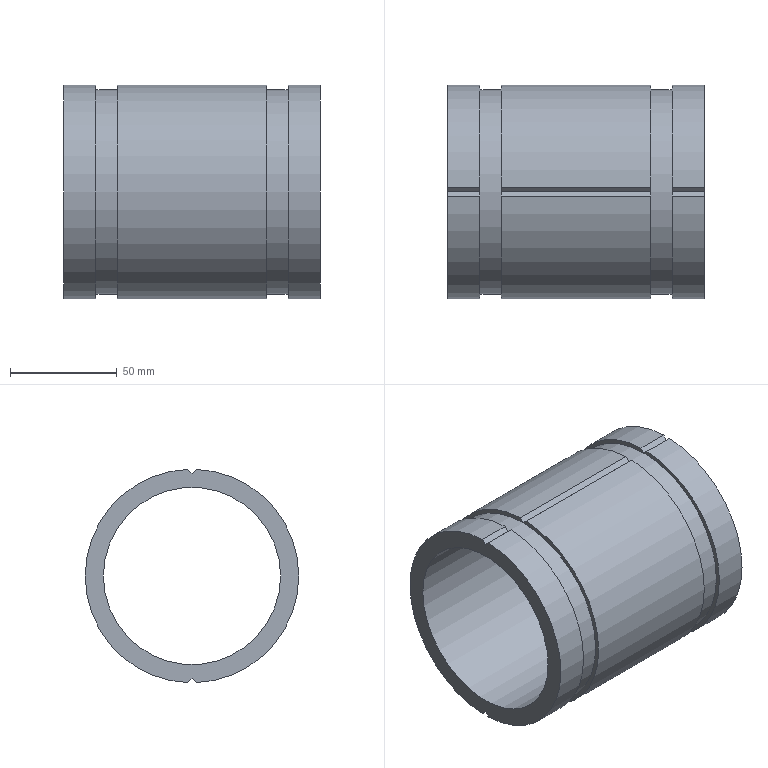Part | NX | features solid 2 | 1 solid | 31 faces | box 120 x 100 x 99.923 mm | volume 280100 mm3 | plane 22 | cylinder 9 | commonest cylinder face diameters 100 x6 96 x2 83 x1
STEP:
#1=CARTESIAN_POINT('',(1975.,798.5,-480.));
#2=VERTEX_POINT('',#1);
#3=CARTESIAN_POINT('',(1975.,840.,-480.));
#4=DIRECTION('',(-1.,0.,0.));
#5=DIRECTION('',(0.,-1.,0.));
#6=AXIS2_PLACEMENT_3D('',#3,#4,#5);
#7=CIRCLE('',#6,41.5);
#8=EDGE_CURVE('',#2,#2,#7,.T.);
#9=ORIENTED_EDGE('',*,*,#8,.T.);
#10=EDGE_LOOP('',(#9));
#11=FACE_BOUND('',#10,.T.);
#12=CARTESIAN_POINT('',(1975.,838.038,-529.962));
#13=VERTEX_POINT('',#12);
#14=CARTESIAN_POINT('',(1975.,840.,-528.));
#15=VERTEX_POINT('',#14);
#16=CARTESIAN_POINT('',(1975.,830.,-538.));
#17=DIRECTION('',(0.,0.7071,0.7071));
#18=VECTOR('',#17,1000.);
#19=LINE('',#16,#18);
#20=EDGE_CURVE('',#13,#15,#19,.T.);
#21=ORIENTED_EDGE('',*,*,#20,.T.);
#22=CARTESIAN_POINT('',(1975.,841.962,-529.962));
#23=VERTEX_POINT('',#22);
#24=CARTESIAN_POINT('',(1975.,840.,-528.));
#25=DIRECTION('',(0.,0.7071,-0.7071));
#26=VECTOR('',#25,1000.);
#27=LINE('',#24,#26);
#28=EDGE_CURVE('',#15,#23,#27,.T.);
#29=ORIENTED_EDGE('',*,*,#28,.T.);
#30=CARTESIAN_POINT('',(1975.,841.962,-430.038));
#31=VERTEX_POINT('',#30);
#32=CARTESIAN_POINT('',(1975.,840.,-480.));
#33=DIRECTION('',(-1.,0.,0.));
#34=DIRECTION('',(0.,-1.,0.));
#35=AXIS2_PLACEMENT_3D('',#32,#33,#34);
#36=CIRCLE('',#35,50.);
#37=EDGE_CURVE('',#31,#23,#36,.T.);
#38=ORIENTED_EDGE('',*,*,#37,.F.);
#39=CARTESIAN_POINT('',(1975.,840.,-432.));
#40=VERTEX_POINT('',#39);
#41=CARTESIAN_POINT('',(1975.,840.,-432.));
#42=DIRECTION('',(0.,0.7071,0.7071));
#43=VECTOR('',#42,1000.);
#44=LINE('',#41,#43);
#45=EDGE_CURVE('',#40,#31,#44,.T.);
#46=ORIENTED_EDGE('',*,*,#45,.F.);
#47=CARTESIAN_POINT('',(1975.,838.038,-430.038));
#48=VERTEX_POINT('',#47);
#49=CARTESIAN_POINT('',(1975.,830.,-422.));
#50=DIRECTION('',(0.,0.7071,-0.7071));
#51=VECTOR('',#50,1000.);
#52=LINE('',#49,#51);
#53=EDGE_CURVE('',#48,#40,#52,.T.);
#54=ORIENTED_EDGE('',*,*,#53,.F.);
#55=CARTESIAN_POINT('',(1975.,840.,-480.));
#56=DIRECTION('',(-1.,0.,0.));
#57=DIRECTION('',(0.,-1.,0.));
#58=AXIS2_PLACEMENT_3D('',#55,#56,#57);
#59=CIRCLE('',#58,50.);
#60=EDGE_CURVE('',#13,#48,#59,.T.);
#61=ORIENTED_EDGE('',*,*,#60,.F.);
#62=EDGE_LOOP('',(#21,#29,#38,#46,#54,#61));
#63=FACE_BOUND('',#62,.T.);
#64=CARTESIAN_POINT('',(1975.,840.,-430.));
#65=DIRECTION('',(1.,0.,0.));
#66=DIRECTION('',(0.,1.,0.));
#67=AXIS2_PLACEMENT_3D('',#64,#65,#66);
#68=PLANE('',#67);
#69=ADVANCED_FACE('',(#11,#63),#68,.T.);
#70=CARTESIAN_POINT('',(1855.,798.5,-480.));
#71=VERTEX_POINT('',#70);
#72=CARTESIAN_POINT('',(1855.,840.,-480.));
#73=DIRECTION('',(-1.,0.,0.));
#74=DIRECTION('',(0.,-1.,0.));
#75=AXIS2_PLACEMENT_3D('',#72,#73,#74);
#76=CIRCLE('',#75,41.5);
#77=EDGE_CURVE('',#71,#71,#76,.T.);
#78=ORIENTED_EDGE('',*,*,#77,.F.);
#79=EDGE_LOOP('',(#78));
#80=FACE_BOUND('',#79,.T.);
#81=CARTESIAN_POINT('',(1855.,841.962,-430.038));
#82=VERTEX_POINT('',#81);
#83=CARTESIAN_POINT('',(1855.,841.962,-529.962));
#84=VERTEX_POINT('',#83);
#85=CARTESIAN_POINT('',(1855.,840.,-480.));
#86=DIRECTION('',(-1.,0.,0.));
#87=DIRECTION('',(0.,-1.,0.));
#88=AXIS2_PLACEMENT_3D('',#85,#86,#87);
#89=CIRCLE('',#88,50.);
#90=EDGE_CURVE('',#82,#84,#89,.T.);
#91=ORIENTED_EDGE('',*,*,#90,.T.);
#92=CARTESIAN_POINT('',(1855.,840.,-528.));
#93=VERTEX_POINT('',#92);
#94=CARTESIAN_POINT('',(1855.,840.,-528.));
#95=DIRECTION('',(0.,0.7071,-0.7071));
#96=VECTOR('',#95,1000.);
#97=LINE('',#94,#96);
#98=EDGE_CURVE('',#93,#84,#97,.T.);
#99=ORIENTED_EDGE('',*,*,#98,.F.);
#100=CARTESIAN_POINT('',(1855.,838.038,-529.962));
#101=VERTEX_POINT('',#100);
#102=CARTESIAN_POINT('',(1855.,830.,-538.));
#103=DIRECTION('',(0.,0.7071,0.7071));
#104=VECTOR('',#103,1000.);
#105=LINE('',#102,#104);
#106=EDGE_CURVE('',#101,#93,#105,.T.);
#107=ORIENTED_EDGE('',*,*,#106,.F.);
#108=CARTESIAN_POINT('',(1855.,838.038,-430.038));
#109=VERTEX_POINT('',#108);
#110=CARTESIAN_POINT('',(1855.,840.,-480.));
#111=DIRECTION('',(-1.,0.,0.));
#112=DIRECTION('',(0.,-1.,0.));
#113=AXIS2_PLACEMENT_3D('',#110,#111,#112);
#114=CIRCLE('',#113,50.);
#115=EDGE_CURVE('',#101,#109,#114,.T.);
#116=ORIENTED_EDGE('',*,*,#115,.T.);
#117=CARTESIAN_POINT('',(1855.,840.,-432.));
#118=VERTEX_POINT('',#117);
#119=CARTESIAN_POINT('',(1855.,830.,-422.));
#120=DIRECTION('',(0.,0.7071,-0.7071));
#121=VECTOR('',#120,1000.);
#122=LINE('',#119,#121);
#123=EDGE_CURVE('',#109,#118,#122,.T.);
#124=ORIENTED_EDGE('',*,*,#123,.T.);
#125=CARTESIAN_POINT('',(1855.,840.,-432.));
#126=DIRECTION('',(0.,0.7071,0.7071));
#127=VECTOR('',#126,1000.);
#128=LINE('',#125,#127);
#129=EDGE_CURVE('',#118,#82,#128,.T.);
#130=ORIENTED_EDGE('',*,*,#129,.T.);
#131=EDGE_LOOP('',(#91,#99,#107,#116,#124,#130));
#132=FACE_BOUND('',#131,.T.);
#133=CARTESIAN_POINT('',(1855.,840.,-438.5));
#134=DIRECTION('',(-1.,0.,0.));
#135=DIRECTION('',(0.,-1.,0.));
#136=AXIS2_PLACEMENT_3D('',#133,#134,#135);
#137=PLANE('',#136);
#138=ADVANCED_FACE('',(#80,#132),#137,.T.);
#139=CARTESIAN_POINT('',(1870.,841.962,-430.038));
#140=VERTEX_POINT('',#139);
#141=CARTESIAN_POINT('',(1870.,841.962,-529.962));
#142=VERTEX_POINT('',#141);
#143=CARTESIAN_POINT('',(1870.,840.,-480.));
#144=DIRECTION('',(-1.,0.,0.));
#145=DIRECTION('',(0.,-1.,0.));
#146=AXIS2_PLACEMENT_3D('',#143,#144,#145);
#147=CIRCLE('',#146,50.);
#148=EDGE_CURVE('',#140,#142,#147,.T.);
#149=ORIENTED_EDGE('',*,*,#148,.T.);
#150=CARTESIAN_POINT('',(2227.4,841.962,-529.962));
#151=DIRECTION('',(-1.,0.,0.));
#152=VECTOR('',#151,1000.);
#153=LINE('',#150,#152);
#154=EDGE_CURVE('',#142,#84,#153,.T.);
#155=ORIENTED_EDGE('',*,*,#154,.T.);
#156=ORIENTED_EDGE('',*,*,#90,.F.);
#157=CARTESIAN_POINT('',(2227.4,841.962,-430.038));
#158=DIRECTION('',(-1.,0.,0.));
#159=VECTOR('',#158,1000.);
#160=LINE('',#157,#159);
#161=EDGE_CURVE('',#140,#82,#160,.T.);
#162=ORIENTED_EDGE('',*,*,#161,.F.);
#163=EDGE_LOOP('',(#149,#155,#156,#162));
#164=FACE_BOUND('',#163,.T.);
#165=CARTESIAN_POINT('',(2227.4,840.,-480.));
#166=DIRECTION('',(-1.,0.,0.));
#167=DIRECTION('',(0.,-1.,0.));
#168=AXIS2_PLACEMENT_3D('',#165,#166,#167);
#169=CYLINDRICAL_SURFACE('',#168,50.);
#170=ADVANCED_FACE('',(#164),#169,.T.);
#171=ORIENTED_EDGE('',*,*,#115,.F.);
#172=CARTESIAN_POINT('',(1870.,838.038,-529.962));
#173=VERTEX_POINT('',#172);
#174=CARTESIAN_POINT('',(2227.4,838.038,-529.962));
#175=DIRECTION('',(-1.,0.,0.));
#176=VECTOR('',#175,1000.);
#177=LINE('',#174,#176);
#178=EDGE_CURVE('',#101,#173,#177,.F.);
#179=ORIENTED_EDGE('',*,*,#178,.T.);
#180=CARTESIAN_POINT('',(1870.,838.038,-430.038));
#181=VERTEX_POINT('',#180);
#182=CARTESIAN_POINT('',(1870.,840.,-480.));
#183=DIRECTION('',(-1.,0.,0.));
#184=DIRECTION('',(0.,-1.,0.));
#185=AXIS2_PLACEMENT_3D('',#182,#183,#184);
#186=CIRCLE('',#185,50.);
#187=EDGE_CURVE('',#173,#181,#186,.T.);
#188=ORIENTED_EDGE('',*,*,#187,.T.);
#189=CARTESIAN_POINT('',(2227.4,838.038,-430.038));
#190=DIRECTION('',(-1.,0.,0.));
#191=VECTOR('',#190,1000.);
#192=LINE('',#189,#191);
#193=EDGE_CURVE('',#109,#181,#192,.F.);
#194=ORIENTED_EDGE('',*,*,#193,.F.);
#195=EDGE_LOOP('',(#171,#179,#188,#194));
#196=FACE_BOUND('',#195,.T.);
#197=CARTESIAN_POINT('',(2227.4,840.,-480.));
#198=DIRECTION('',(-1.,0.,0.));
#199=DIRECTION('',(0.,-1.,0.));
#200=AXIS2_PLACEMENT_3D('',#197,#198,#199);
#201=CYLINDRICAL_SURFACE('',#200,50.);
#202=ADVANCED_FACE('',(#196),#201,.T.);
#203=CARTESIAN_POINT('',(1870.,840.,-432.));
#204=VERTEX_POINT('',#203);
#205=CARTESIAN_POINT('',(1870.,840.,-528.));
#206=VERTEX_POINT('',#205);
#207=CARTESIAN_POINT('',(1870.,840.,-480.));
#208=DIRECTION('',(-1.,0.,0.));
#209=DIRECTION('',(0.,-1.,0.));
#210=AXIS2_PLACEMENT_3D('',#207,#208,#209);
#211=CIRCLE('',#210,48.);
#212=EDGE_CURVE('',#204,#206,#211,.T.);
#213=ORIENTED_EDGE('',*,*,#212,.T.);
#214=CARTESIAN_POINT('',(1870.,791.,-479.));
#215=DIRECTION('',(0.,0.7071,-0.7071));
#216=VECTOR('',#215,1000.);
#217=LINE('',#214,#216);
#218=EDGE_CURVE('',#206,#142,#217,.T.);
#219=ORIENTED_EDGE('',*,*,#218,.T.);
#220=ORIENTED_EDGE('',*,*,#148,.F.);
#221=CARTESIAN_POINT('',(1870.,841.,-431.));
#222=DIRECTION('',(0.,0.7071,0.7071));
#223=VECTOR('',#222,1000.);
#224=LINE('',#221,#223);
#225=EDGE_CURVE('',#204,#140,#224,.T.);
#226=ORIENTED_EDGE('',*,*,#225,.F.);
#227=EDGE_LOOP('',(#213,#219,#220,#226));
#228=FACE_BOUND('',#227,.T.);
#229=CARTESIAN_POINT('',(1870.,840.,-430.));
#230=DIRECTION('',(1.,0.,0.));
#231=DIRECTION('',(0.,1.,0.));
#232=AXIS2_PLACEMENT_3D('',#229,#230,#231);
#233=PLANE('',#232);
#234=ADVANCED_FACE('',(#228),#233,.T.);
#235=ORIENTED_EDGE('',*,*,#187,.F.);
#236=CARTESIAN_POINT('',(1870.,889.,-479.));
#237=DIRECTION('',(0.,0.7071,0.7071));
#238=VECTOR('',#237,1000.);
#239=LINE('',#236,#238);
#240=EDGE_CURVE('',#173,#206,#239,.T.);
#241=ORIENTED_EDGE('',*,*,#240,.T.);
#242=CARTESIAN_POINT('',(1870.,840.,-480.));
#243=DIRECTION('',(-1.,0.,0.));
#244=DIRECTION('',(0.,-1.,0.));
#245=AXIS2_PLACEMENT_3D('',#242,#243,#244);
#246=CIRCLE('',#245,48.);
#247=EDGE_CURVE('',#206,#204,#246,.T.);
#248=ORIENTED_EDGE('',*,*,#247,.T.);
#249=CARTESIAN_POINT('',(1870.,839.,-431.));
#250=DIRECTION('',(0.,0.7071,-0.7071));
#251=VECTOR('',#250,1000.);
#252=LINE('',#249,#251);
#253=EDGE_CURVE('',#181,#204,#252,.T.);
#254=ORIENTED_EDGE('',*,*,#253,.F.);
#255=EDGE_LOOP('',(#235,#241,#248,#254));
#256=FACE_BOUND('',#255,.T.);
#257=CARTESIAN_POINT('',(1870.,840.,-430.));
#258=DIRECTION('',(1.,0.,0.));
#259=DIRECTION('',(0.,1.,0.));
#260=AXIS2_PLACEMENT_3D('',#257,#258,#259);
#261=PLANE('',#260);
#262=ADVANCED_FACE('',(#256),#261,.T.);
#263=CARTESIAN_POINT('',(1880.,841.962,-430.038));
#264=VERTEX_POINT('',#263);
#265=CARTESIAN_POINT('',(1880.,841.962,-529.962));
#266=VERTEX_POINT('',#265);
#267=CARTESIAN_POINT('',(1880.,840.,-480.));
#268=DIRECTION('',(-1.,0.,0.));
#269=DIRECTION('',(0.,-1.,0.));
#270=AXIS2_PLACEMENT_3D('',#267,#268,#269);
#271=CIRCLE('',#270,50.);
#272=EDGE_CURVE('',#264,#266,#271,.T.);
#273=ORIENTED_EDGE('',*,*,#272,.T.);
#274=CARTESIAN_POINT('',(1880.,840.,-528.));
#275=VERTEX_POINT('',#274);
#276=CARTESIAN_POINT('',(1880.,792.,-480.));
#277=DIRECTION('',(0.,-0.7071,0.7071));
#278=VECTOR('',#277,1000.);
#279=LINE('',#276,#278);
#280=EDGE_CURVE('',#266,#275,#279,.T.);
#281=ORIENTED_EDGE('',*,*,#280,.T.);
#282=CARTESIAN_POINT('',(1880.,840.,-432.));
#283=VERTEX_POINT('',#282);
#284=CARTESIAN_POINT('',(1880.,840.,-480.));
#285=DIRECTION('',(-1.,0.,0.));
#286=DIRECTION('',(0.,-1.,0.));
#287=AXIS2_PLACEMENT_3D('',#284,#285,#286);
#288=CIRCLE('',#287,48.);
#289=EDGE_CURVE('',#283,#275,#288,.T.);
#290=ORIENTED_EDGE('',*,*,#289,.F.);
#291=CARTESIAN_POINT('',(1880.,840.,-432.));
#292=DIRECTION('',(0.,-0.7071,-0.7071));
#293=VECTOR('',#292,1000.);
#294=LINE('',#291,#293);
#295=EDGE_CURVE('',#264,#283,#294,.T.);
#296=ORIENTED_EDGE('',*,*,#295,.F.);
#297=EDGE_LOOP('',(#273,#281,#290,#296));
#298=FACE_BOUND('',#297,.T.);
#299=CARTESIAN_POINT('',(1880.,840.,-432.));
#300=DIRECTION('',(-1.,0.,0.));
#301=DIRECTION('',(0.,-1.,0.));
#302=AXIS2_PLACEMENT_3D('',#299,#300,#301);
#303=PLANE('',#302);
#304=ADVANCED_FACE('',(#298),#303,.T.);
#305=CARTESIAN_POINT('',(1880.,840.,-480.));
#306=DIRECTION('',(-1.,0.,0.));
#307=DIRECTION('',(0.,-1.,0.));
#308=AXIS2_PLACEMENT_3D('',#305,#306,#307);
#309=CIRCLE('',#308,48.);
#310=EDGE_CURVE('',#275,#283,#309,.T.);
#311=ORIENTED_EDGE('',*,*,#310,.F.);
#312=CARTESIAN_POINT('',(1880.,838.038,-529.962));
#313=VERTEX_POINT('',#312);
#314=CARTESIAN_POINT('',(1880.,888.,-480.));
#315=DIRECTION('',(0.,-0.7071,-0.7071));
#316=VECTOR('',#315,1000.);
#317=LINE('',#314,#316);
#318=EDGE_CURVE('',#275,#313,#317,.T.);
#319=ORIENTED_EDGE('',*,*,#318,.T.);
#320=CARTESIAN_POINT('',(1880.,838.038,-430.038));
#321=VERTEX_POINT('',#320);
#322=CARTESIAN_POINT('',(1880.,840.,-480.));
#323=DIRECTION('',(-1.,0.,0.));
#324=DIRECTION('',(0.,-1.,0.));
#325=AXIS2_PLACEMENT_3D('',#322,#323,#324);
#326=CIRCLE('',#325,50.);
#327=EDGE_CURVE('',#313,#321,#326,.T.);
#328=ORIENTED_EDGE('',*,*,#327,.T.);
#329=CARTESIAN_POINT('',(1880.,840.,-432.));
#330=DIRECTION('',(0.,-0.7071,0.7071));
#331=VECTOR('',#330,1000.);
#332=LINE('',#329,#331);
#333=EDGE_CURVE('',#283,#321,#332,.T.);
#334=ORIENTED_EDGE('',*,*,#333,.F.);
#335=EDGE_LOOP('',(#311,#319,#328,#334));
#336=FACE_BOUND('',#335,.T.);
#337=CARTESIAN_POINT('',(1880.,840.,-432.));
#338=DIRECTION('',(-1.,0.,0.));
#339=DIRECTION('',(0.,-1.,0.));
#340=AXIS2_PLACEMENT_3D('',#337,#338,#339);
#341=PLANE('',#340);
#342=ADVANCED_FACE('',(#336),#341,.T.);
#343=CARTESIAN_POINT('',(1950.,841.962,-430.038));
#344=VERTEX_POINT('',#343);
#345=CARTESIAN_POINT('',(1950.,841.962,-529.962));
#346=VERTEX_POINT('',#345);
#347=CARTESIAN_POINT('',(1950.,840.,-480.));
#348=DIRECTION('',(-1.,0.,0.));
#349=DIRECTION('',(0.,-1.,0.));
#350=AXIS2_PLACEMENT_3D('',#347,#348,#349);
#351=CIRCLE('',#350,50.);
#352=EDGE_CURVE('',#344,#346,#351,.T.);
#353=ORIENTED_EDGE('',*,*,#352,.T.);
#354=CARTESIAN_POINT('',(2227.4,841.962,-529.962));
#355=DIRECTION('',(-1.,0.,0.));
#356=VECTOR('',#355,1000.);
#357=LINE('',#354,#356);
#358=EDGE_CURVE('',#346,#266,#357,.T.);
#359=ORIENTED_EDGE('',*,*,#358,.T.);
#360=ORIENTED_EDGE('',*,*,#272,.F.);
#361=CARTESIAN_POINT('',(2227.4,841.962,-430.038));
#362=DIRECTION('',(-1.,0.,0.));
#363=VECTOR('',#362,1000.);
#364=LINE('',#361,#363);
#365=EDGE_CURVE('',#344,#264,#364,.T.);
#366=ORIENTED_EDGE('',*,*,#365,.F.);
#367=EDGE_LOOP('',(#353,#359,#360,#366));
#368=FACE_BOUND('',#367,.T.);
#369=CARTESIAN_POINT('',(2227.4,840.,-480.));
#370=DIRECTION('',(-1.,0.,0.));
#371=DIRECTION('',(0.,-1.,0.));
#372=AXIS2_PLACEMENT_3D('',#369,#370,#371);
#373=CYLINDRICAL_SURFACE('',#372,50.);
#374=ADVANCED_FACE('',(#368),#373,.T.);
#375=ORIENTED_EDGE('',*,*,#327,.F.);
#376=CARTESIAN_POINT('',(1950.,838.038,-529.962));
#377=VERTEX_POINT('',#376);
#378=CARTESIAN_POINT('',(2227.4,838.038,-529.962));
#379=DIRECTION('',(-1.,0.,0.));
#380=VECTOR('',#379,1000.);
#381=LINE('',#378,#380);
#382=EDGE_CURVE('',#313,#377,#381,.F.);
#383=ORIENTED_EDGE('',*,*,#382,.T.);
#384=CARTESIAN_POINT('',(1950.,838.038,-430.038));
#385=VERTEX_POINT('',#384);
#386=CARTESIAN_POINT('',(1950.,840.,-480.));
#387=DIRECTION('',(-1.,0.,0.));
#388=DIRECTION('',(0.,-1.,0.));
#389=AXIS2_PLACEMENT_3D('',#386,#387,#388);
#390=CIRCLE('',#389,50.);
#391=EDGE_CURVE('',#377,#385,#390,.T.);
#392=ORIENTED_EDGE('',*,*,#391,.T.);
#393=CARTESIAN_POINT('',(2227.4,838.038,-430.038));
#394=DIRECTION('',(-1.,0.,0.));
#395=VECTOR('',#394,1000.);
#396=LINE('',#393,#395);
#397=EDGE_CURVE('',#321,#385,#396,.F.);
#398=ORIENTED_EDGE('',*,*,#397,.F.);
#399=EDGE_LOOP('',(#375,#383,#392,#398));
#400=FACE_BOUND('',#399,.T.);
#401=CARTESIAN_POINT('',(2227.4,840.,-480.));
#402=DIRECTION('',(-1.,0.,0.));
#403=DIRECTION('',(0.,-1.,0.));
#404=AXIS2_PLACEMENT_3D('',#401,#402,#403);
#405=CYLINDRICAL_SURFACE('',#404,50.);
#406=ADVANCED_FACE('',(#400),#405,.T.);
#407=CARTESIAN_POINT('',(1950.,840.,-432.));
#408=VERTEX_POINT('',#407);
#409=CARTESIAN_POINT('',(1950.,840.,-528.));
#410=VERTEX_POINT('',#409);
#411=CARTESIAN_POINT('',(1950.,840.,-480.));
#412=DIRECTION('',(-1.,0.,0.));
#413=DIRECTION('',(0.,-1.,0.));
#414=AXIS2_PLACEMENT_3D('',#411,#412,#413);
#415=CIRCLE('',#414,48.);
#416=EDGE_CURVE('',#408,#410,#415,.T.);
#417=ORIENTED_EDGE('',*,*,#416,.T.);
#418=CARTESIAN_POINT('',(1950.,791.,-479.));
#419=DIRECTION('',(0.,0.7071,-0.7071));
#420=VECTOR('',#419,1000.);
#421=LINE('',#418,#420);
#422=EDGE_CURVE('',#410,#346,#421,.T.);
#423=ORIENTED_EDGE('',*,*,#422,.T.);
#424=ORIENTED_EDGE('',*,*,#352,.F.);
#425=CARTESIAN_POINT('',(1950.,841.,-431.));
#426=DIRECTION('',(0.,0.7071,0.7071));
#427=VECTOR('',#426,1000.);
#428=LINE('',#425,#427);
#429=EDGE_CURVE('',#408,#344,#428,.T.);
#430=ORIENTED_EDGE('',*,*,#429,.F.);
#431=EDGE_LOOP('',(#417,#423,#424,#430));
#432=FACE_BOUND('',#431,.T.);
#433=CARTESIAN_POINT('',(1950.,840.,-430.));
#434=DIRECTION('',(1.,0.,0.));
#435=DIRECTION('',(0.,1.,0.));
#436=AXIS2_PLACEMENT_3D('',#433,#434,#435);
#437=PLANE('',#436);
#438=ADVANCED_FACE('',(#432),#437,.T.);
#439=ORIENTED_EDGE('',*,*,#391,.F.);
#440=CARTESIAN_POINT('',(1950.,889.,-479.));
#441=DIRECTION('',(0.,0.7071,0.7071));
#442=VECTOR('',#441,1000.);
#443=LINE('',#440,#442);
#444=EDGE_CURVE('',#377,#410,#443,.T.);
#445=ORIENTED_EDGE('',*,*,#444,.T.);
#446=CARTESIAN_POINT('',(1950.,840.,-480.));
#447=DIRECTION('',(-1.,0.,0.));
#448=DIRECTION('',(0.,-1.,0.));
#449=AXIS2_PLACEMENT_3D('',#446,#447,#448);
#450=CIRCLE('',#449,48.);
#451=EDGE_CURVE('',#410,#408,#450,.T.);
#452=ORIENTED_EDGE('',*,*,#451,.T.);
#453=CARTESIAN_POINT('',(1950.,839.,-431.));
#454=DIRECTION('',(0.,0.7071,-0.7071));
#455=VECTOR('',#454,1000.);
#456=LINE('',#453,#455);
#457=EDGE_CURVE('',#385,#408,#456,.T.);
#458=ORIENTED_EDGE('',*,*,#457,.F.);
#459=EDGE_LOOP('',(#439,#445,#452,#458));
#460=FACE_BOUND('',#459,.T.);
#461=CARTESIAN_POINT('',(1950.,840.,-430.));
#462=DIRECTION('',(1.,0.,0.));
#463=DIRECTION('',(0.,1.,0.));
#464=AXIS2_PLACEMENT_3D('',#461,#462,#463);
#465=PLANE('',#464);
#466=ADVANCED_FACE('',(#460),#465,.T.);
#467=CARTESIAN_POINT('',(1960.,841.962,-430.038));
#468=VERTEX_POINT('',#467);
#469=CARTESIAN_POINT('',(1960.,841.962,-529.962));
#470=VERTEX_POINT('',#469);
#471=CARTESIAN_POINT('',(1960.,840.,-480.));
#472=DIRECTION('',(-1.,0.,0.));
#473=DIRECTION('',(0.,-1.,0.));
#474=AXIS2_PLACEMENT_3D('',#471,#472,#473);
#475=CIRCLE('',#474,50.);
#476=EDGE_CURVE('',#468,#470,#475,.T.);
#477=ORIENTED_EDGE('',*,*,#476,.T.);
#478=CARTESIAN_POINT('',(1960.,840.,-528.));
#479=VERTEX_POINT('',#478);
#480=CARTESIAN_POINT('',(1960.,792.,-480.));
#481=DIRECTION('',(0.,-0.7071,0.7071));
#482=VECTOR('',#481,1000.);
#483=LINE('',#480,#482);
#484=EDGE_CURVE('',#470,#479,#483,.T.);
#485=ORIENTED_EDGE('',*,*,#484,.T.);
#486=CARTESIAN_POINT('',(1960.,840.,-432.));
#487=VERTEX_POINT('',#486);
#488=CARTESIAN_POINT('',(1960.,840.,-480.));
#489=DIRECTION('',(-1.,0.,0.));
#490=DIRECTION('',(0.,-1.,0.));
#491=AXIS2_PLACEMENT_3D('',#488,#489,#490);
#492=CIRCLE('',#491,48.);
#493=EDGE_CURVE('',#487,#479,#492,.T.);
#494=ORIENTED_EDGE('',*,*,#493,.F.);
#495=CARTESIAN_POINT('',(1960.,840.,-432.));
#496=DIRECTION('',(0.,-0.7071,-0.7071));
#497=VECTOR('',#496,1000.);
#498=LINE('',#495,#497);
#499=EDGE_CURVE('',#468,#487,#498,.T.);
#500=ORIENTED_EDGE('',*,*,#499,.F.);
#501=EDGE_LOOP('',(#477,#485,#494,#500));
#502=FACE_BOUND('',#501,.T.);
#503=CARTESIAN_POINT('',(1960.,840.,-432.));
#504=DIRECTION('',(-1.,0.,0.));
#505=DIRECTION('',(0.,-1.,0.));
#506=AXIS2_PLACEMENT_3D('',#503,#504,#505);
#507=PLANE('',#506);
#508=ADVANCED_FACE('',(#502),#507,.T.);
#509=CARTESIAN_POINT('',(1960.,840.,-480.));
#510=DIRECTION('',(-1.,0.,0.));
#511=DIRECTION('',(0.,-1.,0.));
#512=AXIS2_PLACEMENT_3D('',#509,#510,#511);
#513=CIRCLE('',#512,48.);
#514=EDGE_CURVE('',#479,#487,#513,.T.);
#515=ORIENTED_EDGE('',*,*,#514,.F.);
#516=CARTESIAN_POINT('',(1960.,838.038,-529.962));
#517=VERTEX_POINT('',#516);
#518=CARTESIAN_POINT('',(1960.,888.,-480.));
#519=DIRECTION('',(0.,-0.7071,-0.7071));
#520=VECTOR('',#519,1000.);
#521=LINE('',#518,#520);
#522=EDGE_CURVE('',#479,#517,#521,.T.);
#523=ORIENTED_EDGE('',*,*,#522,.T.);
#524=CARTESIAN_POINT('',(1960.,838.038,-430.038));
#525=VERTEX_POINT('',#524);
#526=CARTESIAN_POINT('',(1960.,840.,-480.));
#527=DIRECTION('',(-1.,0.,0.));
#528=DIRECTION('',(0.,-1.,0.));
#529=AXIS2_PLACEMENT_3D('',#526,#527,#528);
#530=CIRCLE('',#529,50.);
#531=EDGE_CURVE('',#517,#525,#530,.T.);
#532=ORIENTED_EDGE('',*,*,#531,.T.);
#533=CARTESIAN_POINT('',(1960.,840.,-432.));
#534=DIRECTION('',(0.,-0.7071,0.7071));
#535=VECTOR('',#534,1000.);
#536=LINE('',#533,#535);
#537=EDGE_CURVE('',#487,#525,#536,.T.);
#538=ORIENTED_EDGE('',*,*,#537,.F.);
#539=EDGE_LOOP('',(#515,#523,#532,#538));
#540=FACE_BOUND('',#539,.T.);
#541=CARTESIAN_POINT('',(1960.,840.,-432.));
#542=DIRECTION('',(-1.,0.,0.));
#543=DIRECTION('',(0.,-1.,0.));
#544=AXIS2_PLACEMENT_3D('',#541,#542,#543);
#545=PLANE('',#544);
#546=ADVANCED_FACE('',(#540),#545,.T.);
#547=ORIENTED_EDGE('',*,*,#37,.T.);
#548=CARTESIAN_POINT('',(2227.4,841.962,-529.962));
#549=DIRECTION('',(-1.,0.,0.));
#550=VECTOR('',#549,1000.);
#551=LINE('',#548,#550);
#552=EDGE_CURVE('',#23,#470,#551,.T.);
#553=ORIENTED_EDGE('',*,*,#552,.T.);
#554=ORIENTED_EDGE('',*,*,#476,.F.);
#555=CARTESIAN_POINT('',(2227.4,841.962,-430.038));
#556=DIRECTION('',(-1.,0.,0.));
#557=VECTOR('',#556,1000.);
#558=LINE('',#555,#557);
#559=EDGE_CURVE('',#31,#468,#558,.T.);
#560=ORIENTED_EDGE('',*,*,#559,.F.);
#561=EDGE_LOOP('',(#547,#553,#554,#560));
#562=FACE_BOUND('',#561,.T.);
#563=CARTESIAN_POINT('',(2227.4,840.,-480.));
#564=DIRECTION('',(-1.,0.,0.));
#565=DIRECTION('',(0.,-1.,0.));
#566=AXIS2_PLACEMENT_3D('',#563,#564,#565);
#567=CYLINDRICAL_SURFACE('',#566,50.);
#568=ADVANCED_FACE('',(#562),#567,.T.);
#569=ORIENTED_EDGE('',*,*,#531,.F.);
#570=CARTESIAN_POINT('',(2227.4,838.038,-529.962));
#571=DIRECTION('',(-1.,0.,0.));
#572=VECTOR('',#571,1000.);
#573=LINE('',#570,#572);
#574=EDGE_CURVE('',#517,#13,#573,.F.);
#575=ORIENTED_EDGE('',*,*,#574,.T.);
#576=ORIENTED_EDGE('',*,*,#60,.T.);
#577=CARTESIAN_POINT('',(2227.4,838.038,-430.038));
#578=DIRECTION('',(-1.,0.,0.));
#579=VECTOR('',#578,1000.);
#580=LINE('',#577,#579);
#581=EDGE_CURVE('',#525,#48,#580,.F.);
#582=ORIENTED_EDGE('',*,*,#581,.F.);
#583=EDGE_LOOP('',(#569,#575,#576,#582));
#584=FACE_BOUND('',#583,.T.);
#585=CARTESIAN_POINT('',(2227.4,840.,-480.));
#586=DIRECTION('',(-1.,0.,0.));
#587=DIRECTION('',(0.,-1.,0.));
#588=AXIS2_PLACEMENT_3D('',#585,#586,#587);
#589=CYLINDRICAL_SURFACE('',#588,50.);
#590=ADVANCED_FACE('',(#584),#589,.T.);
#591=ORIENTED_EDGE('',*,*,#8,.F.);
#592=EDGE_LOOP('',(#591));
#593=FACE_BOUND('',#592,.T.);
#594=ORIENTED_EDGE('',*,*,#77,.T.);
#595=EDGE_LOOP('',(#594));
#596=FACE_BOUND('',#595,.T.);
#597=CARTESIAN_POINT('',(2227.4,840.,-480.));
#598=DIRECTION('',(-1.,0.,0.));
#599=DIRECTION('',(0.,-1.,0.));
#600=AXIS2_PLACEMENT_3D('',#597,#598,#599);
#601=CYLINDRICAL_SURFACE('',#600,41.5);
#602=ADVANCED_FACE('',(#593,#596),#601,.F.);
#603=ORIENTED_EDGE('',*,*,#289,.T.);
#604=ORIENTED_EDGE('',*,*,#310,.T.);
#605=EDGE_LOOP('',(#603,#604));
#606=FACE_BOUND('',#605,.T.);
#607=ORIENTED_EDGE('',*,*,#212,.F.);
#608=ORIENTED_EDGE('',*,*,#247,.F.);
#609=EDGE_LOOP('',(#607,#608));
#610=FACE_BOUND('',#609,.T.);
#611=CARTESIAN_POINT('',(2227.4,840.,-480.));
#612=DIRECTION('',(-1.,0.,0.));
#613=DIRECTION('',(0.,-1.,0.));
#614=AXIS2_PLACEMENT_3D('',#611,#612,#613);
#615=CYLINDRICAL_SURFACE('',#614,48.);
#616=ADVANCED_FACE('',(#606,#610),#615,.T.);
#617=ORIENTED_EDGE('',*,*,#493,.T.);
#618=ORIENTED_EDGE('',*,*,#514,.T.);
#619=EDGE_LOOP('',(#617,#618));
#620=FACE_BOUND('',#619,.T.);
#621=ORIENTED_EDGE('',*,*,#416,.F.);
#622=ORIENTED_EDGE('',*,*,#451,.F.);
#623=EDGE_LOOP('',(#621,#622));
#624=FACE_BOUND('',#623,.T.);
#625=CARTESIAN_POINT('',(2227.4,840.,-480.));
#626=DIRECTION('',(-1.,0.,0.));
#627=DIRECTION('',(0.,-1.,0.));
#628=AXIS2_PLACEMENT_3D('',#625,#626,#627);
#629=CYLINDRICAL_SURFACE('',#628,48.);
#630=ADVANCED_FACE('',(#620,#624),#629,.T.);
#631=ORIENTED_EDGE('',*,*,#499,.T.);
#632=CARTESIAN_POINT('',(1855.,840.,-432.));
#633=DIRECTION('',(1.,0.,0.));
#634=VECTOR('',#633,1000.);
#635=LINE('',#632,#634);
#636=EDGE_CURVE('',#487,#40,#635,.T.);
#637=ORIENTED_EDGE('',*,*,#636,.T.);
#638=ORIENTED_EDGE('',*,*,#45,.T.);
#639=ORIENTED_EDGE('',*,*,#559,.T.);
#640=EDGE_LOOP('',(#631,#637,#638,#639));
#641=FACE_BOUND('',#640,.T.);
#642=CARTESIAN_POINT('',(1855.,840.,-432.));
#643=DIRECTION('',(0.,0.7071,-0.7071));
#644=DIRECTION('',(0.,0.7071,0.7071));
#645=AXIS2_PLACEMENT_3D('',#642,#643,#644);
#646=PLANE('',#645);
#647=ADVANCED_FACE('',(#641),#646,.F.);
#648=ORIENTED_EDGE('',*,*,#537,.T.);
#649=ORIENTED_EDGE('',*,*,#581,.T.);
#650=ORIENTED_EDGE('',*,*,#53,.T.);
#651=ORIENTED_EDGE('',*,*,#636,.F.);
#652=EDGE_LOOP('',(#648,#649,#650,#651));
#653=FACE_BOUND('',#652,.T.);
#654=CARTESIAN_POINT('',(1855.,830.,-422.));
#655=DIRECTION('',(0.,-0.7071,-0.7071));
#656=DIRECTION('',(0.,0.7071,-0.7071));
#657=AXIS2_PLACEMENT_3D('',#654,#655,#656);
#658=PLANE('',#657);
#659=ADVANCED_FACE('',(#653),#658,.F.);
#660=ORIENTED_EDGE('',*,*,#295,.T.);
#661=CARTESIAN_POINT('',(1855.,840.,-432.));
#662=DIRECTION('',(1.,0.,0.));
#663=VECTOR('',#662,1000.);
#664=LINE('',#661,#663);
#665=EDGE_CURVE('',#283,#408,#664,.T.);
#666=ORIENTED_EDGE('',*,*,#665,.T.);
#667=ORIENTED_EDGE('',*,*,#429,.T.);
#668=ORIENTED_EDGE('',*,*,#365,.T.);
#669=EDGE_LOOP('',(#660,#666,#667,#668));
#670=FACE_BOUND('',#669,.T.);
#671=CARTESIAN_POINT('',(1855.,840.,-432.));
#672=DIRECTION('',(0.,0.7071,-0.7071));
#673=DIRECTION('',(0.,0.7071,0.7071));
#674=AXIS2_PLACEMENT_3D('',#671,#672,#673);
#675=PLANE('',#674);
#676=ADVANCED_FACE('',(#670),#675,.F.);
#677=ORIENTED_EDGE('',*,*,#333,.T.);
#678=ORIENTED_EDGE('',*,*,#397,.T.);
#679=ORIENTED_EDGE('',*,*,#457,.T.);
#680=ORIENTED_EDGE('',*,*,#665,.F.);
#681=EDGE_LOOP('',(#677,#678,#679,#680));
#682=FACE_BOUND('',#681,.T.);
#683=CARTESIAN_POINT('',(1855.,830.,-422.));
#684=DIRECTION('',(0.,-0.7071,-0.7071));
#685=DIRECTION('',(0.,0.7071,-0.7071));
#686=AXIS2_PLACEMENT_3D('',#683,#684,#685);
#687=PLANE('',#686);
#688=ADVANCED_FACE('',(#682),#687,.F.);
#689=ORIENTED_EDGE('',*,*,#193,.T.);
#690=ORIENTED_EDGE('',*,*,#253,.T.);
#691=CARTESIAN_POINT('',(1855.,840.,-432.));
#692=DIRECTION('',(1.,0.,0.));
#693=VECTOR('',#692,1000.);
#694=LINE('',#691,#693);
#695=EDGE_CURVE('',#118,#204,#694,.T.);
#696=ORIENTED_EDGE('',*,*,#695,.F.);
#697=ORIENTED_EDGE('',*,*,#123,.F.);
#698=EDGE_LOOP('',(#689,#690,#696,#697));
#699=FACE_BOUND('',#698,.T.);
#700=CARTESIAN_POINT('',(1855.,830.,-422.));
#701=DIRECTION('',(0.,-0.7071,-0.7071));
#702=DIRECTION('',(0.,0.7071,-0.7071));
#703=AXIS2_PLACEMENT_3D('',#700,#701,#702);
#704=PLANE('',#703);
#705=ADVANCED_FACE('',(#699),#704,.F.);
#706=ORIENTED_EDGE('',*,*,#161,.T.);
#707=ORIENTED_EDGE('',*,*,#129,.F.);
#708=ORIENTED_EDGE('',*,*,#695,.T.);
#709=ORIENTED_EDGE('',*,*,#225,.T.);
#710=EDGE_LOOP('',(#706,#707,#708,#709));
#711=FACE_BOUND('',#710,.T.);
#712=CARTESIAN_POINT('',(1855.,840.,-432.));
#713=DIRECTION('',(0.,0.7071,-0.7071));
#714=DIRECTION('',(0.,0.7071,0.7071));
#715=AXIS2_PLACEMENT_3D('',#712,#713,#714);
#716=PLANE('',#715);
#717=ADVANCED_FACE('',(#711),#716,.F.);
#718=CARTESIAN_POINT('',(1855.,840.,-528.));
#719=DIRECTION('',(1.,0.,0.));
#720=VECTOR('',#719,1000.);
#721=LINE('',#718,#720);
#722=EDGE_CURVE('',#479,#15,#721,.T.);
#723=ORIENTED_EDGE('',*,*,#722,.T.);
#724=ORIENTED_EDGE('',*,*,#20,.F.);
#725=ORIENTED_EDGE('',*,*,#574,.F.);
#726=ORIENTED_EDGE('',*,*,#522,.F.);
#727=EDGE_LOOP('',(#723,#724,#725,#726));
#728=FACE_BOUND('',#727,.T.);
#729=CARTESIAN_POINT('',(1855.,830.,-538.));
#730=DIRECTION('',(0.,0.7071,-0.7071));
#731=DIRECTION('',(0.,0.7071,0.7071));
#732=AXIS2_PLACEMENT_3D('',#729,#730,#731);
#733=PLANE('',#732);
#734=ADVANCED_FACE('',(#728),#733,.T.);
#735=ORIENTED_EDGE('',*,*,#552,.F.);
#736=ORIENTED_EDGE('',*,*,#28,.F.);
#737=ORIENTED_EDGE('',*,*,#722,.F.);
#738=ORIENTED_EDGE('',*,*,#484,.F.);
#739=EDGE_LOOP('',(#735,#736,#737,#738));
#740=FACE_BOUND('',#739,.T.);
#741=CARTESIAN_POINT('',(1855.,840.,-528.));
#742=DIRECTION('',(0.,-0.7071,-0.7071));
#743=DIRECTION('',(0.,0.7071,-0.7071));
#744=AXIS2_PLACEMENT_3D('',#741,#742,#743);
#745=PLANE('',#744);
#746=ADVANCED_FACE('',(#740),#745,.T.);
#747=CARTESIAN_POINT('',(1855.,840.,-528.));
#748=DIRECTION('',(1.,0.,0.));
#749=VECTOR('',#748,1000.);
#750=LINE('',#747,#749);
#751=EDGE_CURVE('',#275,#410,#750,.T.);
#752=ORIENTED_EDGE('',*,*,#751,.T.);
#753=ORIENTED_EDGE('',*,*,#444,.F.);
#754=ORIENTED_EDGE('',*,*,#382,.F.);
#755=ORIENTED_EDGE('',*,*,#318,.F.);
#756=EDGE_LOOP('',(#752,#753,#754,#755));
#757=FACE_BOUND('',#756,.T.);
#758=CARTESIAN_POINT('',(1855.,830.,-538.));
#759=DIRECTION('',(0.,0.7071,-0.7071));
#760=DIRECTION('',(0.,0.7071,0.7071));
#761=AXIS2_PLACEMENT_3D('',#758,#759,#760);
#762=PLANE('',#761);
#763=ADVANCED_FACE('',(#757),#762,.T.);
#764=ORIENTED_EDGE('',*,*,#358,.F.);
#765=ORIENTED_EDGE('',*,*,#422,.F.);
#766=ORIENTED_EDGE('',*,*,#751,.F.);
#767=ORIENTED_EDGE('',*,*,#280,.F.);
#768=EDGE_LOOP('',(#764,#765,#766,#767));
#769=FACE_BOUND('',#768,.T.);
#770=CARTESIAN_POINT('',(1855.,840.,-528.));
#771=DIRECTION('',(0.,-0.7071,-0.7071));
#772=DIRECTION('',(0.,0.7071,-0.7071));
#773=AXIS2_PLACEMENT_3D('',#770,#771,#772);
#774=PLANE('',#773);
#775=ADVANCED_FACE('',(#769),#774,.T.);
#776=ORIENTED_EDGE('',*,*,#218,.F.);
#777=CARTESIAN_POINT('',(1855.,840.,-528.));
#778=DIRECTION('',(1.,0.,0.));
#779=VECTOR('',#778,1000.);
#780=LINE('',#777,#779);
#781=EDGE_CURVE('',#93,#206,#780,.T.);
#782=ORIENTED_EDGE('',*,*,#781,.F.);
#783=ORIENTED_EDGE('',*,*,#98,.T.);
#784=ORIENTED_EDGE('',*,*,#154,.F.);
#785=EDGE_LOOP('',(#776,#782,#783,#784));
#786=FACE_BOUND('',#785,.T.);
#787=CARTESIAN_POINT('',(1855.,840.,-528.));
#788=DIRECTION('',(0.,-0.7071,-0.7071));
#789=DIRECTION('',(0.,0.7071,-0.7071));
#790=AXIS2_PLACEMENT_3D('',#787,#788,#789);
#791=PLANE('',#790);
#792=ADVANCED_FACE('',(#786),#791,.T.);
#793=ORIENTED_EDGE('',*,*,#106,.T.);
#794=ORIENTED_EDGE('',*,*,#781,.T.);
#795=ORIENTED_EDGE('',*,*,#240,.F.);
#796=ORIENTED_EDGE('',*,*,#178,.F.);
#797=EDGE_LOOP('',(#793,#794,#795,#796));
#798=FACE_BOUND('',#797,.T.);
#799=CARTESIAN_POINT('',(1855.,830.,-538.));
#800=DIRECTION('',(0.,0.7071,-0.7071));
#801=DIRECTION('',(0.,0.7071,0.7071));
#802=AXIS2_PLACEMENT_3D('',#799,#800,#801);
#803=PLANE('',#802);
#804=ADVANCED_FACE('',(#798),#803,.T.);
#805=CLOSED_SHELL('',(#69,#138,#170,#202,#234,#262,#304,#342,#374,#406,#438,#466,#508,#546,#568,#590,#602,#616,#630,#647,#659,#676,#688,#705,#717,#734,#746,#763,#775,#792,#804));
#806=MANIFOLD_SOLID_BREP('',#805);
#807=(LENGTH_UNIT()NAMED_UNIT(*)SI_UNIT(.MILLI.,.METRE.));
#808=UNCERTAINTY_MEASURE_WITH_UNIT(LENGTH_MEASURE(0.00001),#807,'','');
#809=(NAMED_UNIT(*)PLANE_ANGLE_UNIT()SI_UNIT($,.RADIAN.));
#810=(NAMED_UNIT(*)SI_UNIT($,.STERADIAN.)SOLID_ANGLE_UNIT());
#811=(GEOMETRIC_REPRESENTATION_CONTEXT(3)GLOBAL_UNCERTAINTY_ASSIGNED_CONTEXT((#808))GLOBAL_UNIT_ASSIGNED_CONTEXT((#807,#809,#810))REPRESENTATION_CONTEXT('',''));
#812=ADVANCED_BREP_SHAPE_REPRESENTATION('',(#806),#811);